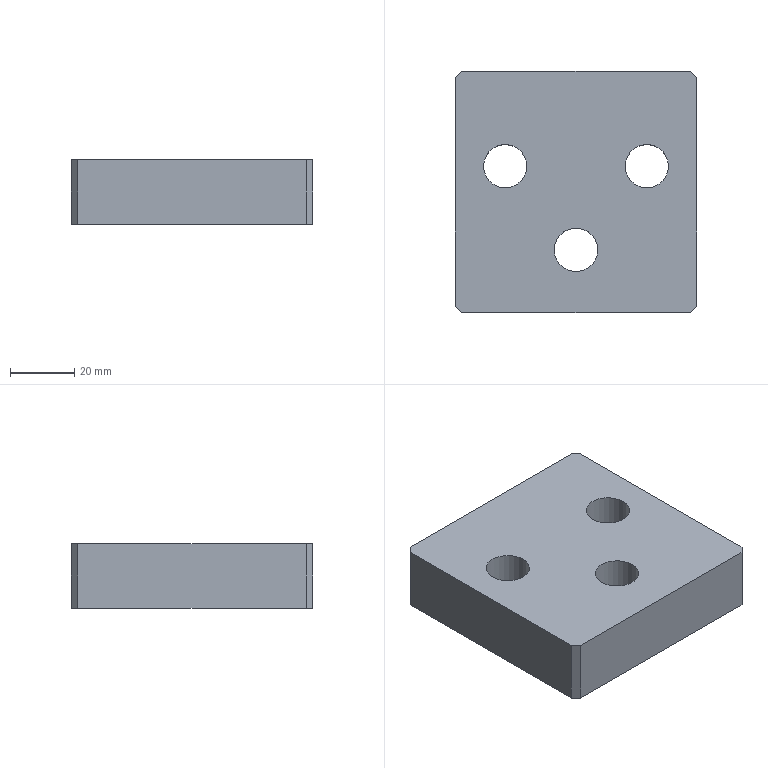Part | STEP file | lll_id1918_x_t | 1 solid | 13 faces | box 75 x 75 x 20 mm | volume 103740 mm3 | plane 10 | cylinder 3 | commonest cylinder face diameters 13.509 x3
STEP:
#1=CARTESIAN_POINT('',(3864.435,-427.,-98.5));
#2=VERTEX_POINT('',#1);
#3=CARTESIAN_POINT('',(3935.435,-427.,-98.5));
#4=VERTEX_POINT('',#3);
#5=CARTESIAN_POINT('',(3873.935,-427.,-98.5));
#6=DIRECTION('',(1.,0.,0.));
#7=VECTOR('',#6,1.);
#8=LINE('',#5,#7);
#9=EDGE_CURVE('',#2,#4,#8,.T.);
#10=ORIENTED_EDGE('',*,*,#9,.T.);
#11=CARTESIAN_POINT('',(3935.435,-427.,-78.5));
#12=VERTEX_POINT('',#11);
#13=CARTESIAN_POINT('',(3935.435,-427.,-78.5));
#14=DIRECTION('',(0.,0.,1.));
#15=VECTOR('',#14,1.);
#16=LINE('',#13,#15);
#17=EDGE_CURVE('',#4,#12,#16,.T.);
#18=ORIENTED_EDGE('',*,*,#17,.T.);
#19=CARTESIAN_POINT('',(3864.435,-427.,-78.5));
#20=VERTEX_POINT('',#19);
#21=CARTESIAN_POINT('',(3873.935,-427.,-78.5));
#22=DIRECTION('',(1.,0.,0.));
#23=VECTOR('',#22,1.);
#24=LINE('',#21,#23);
#25=EDGE_CURVE('',#20,#12,#24,.T.);
#26=ORIENTED_EDGE('',*,*,#25,.F.);
#27=CARTESIAN_POINT('',(3864.435,-427.,-78.5));
#28=DIRECTION('',(0.,0.,-1.));
#29=VECTOR('',#28,1.);
#30=LINE('',#27,#29);
#31=EDGE_CURVE('',#20,#2,#30,.T.);
#32=ORIENTED_EDGE('',*,*,#31,.T.);
#33=EDGE_LOOP('',(#10,#18,#26,#32));
#34=FACE_OUTER_BOUND('',#33,.T.);
#35=CARTESIAN_POINT('',(3873.935,-427.,-78.5));
#36=DIRECTION('',(0.,1.,0.));
#37=DIRECTION('',(0.,0.,1.));
#38=AXIS2_PLACEMENT_3D('',#35,#36,#37);
#39=PLANE('',#38);
#40=ADVANCED_FACE('',(#34),#39,.F.);
#41=CARTESIAN_POINT('',(3862.435,-354.,-78.5));
#42=VERTEX_POINT('',#41);
#43=CARTESIAN_POINT('',(3862.435,-425.,-78.5));
#44=VERTEX_POINT('',#43);
#45=CARTESIAN_POINT('',(3862.435,-362.5,-78.5));
#46=DIRECTION('',(0.,-1.,0.));
#47=VECTOR('',#46,1.);
#48=LINE('',#45,#47);
#49=EDGE_CURVE('',#42,#44,#48,.T.);
#50=ORIENTED_EDGE('',*,*,#49,.F.);
#51=CARTESIAN_POINT('',(3862.435,-354.,-98.5));
#52=VERTEX_POINT('',#51);
#53=CARTESIAN_POINT('',(3862.435,-354.,-78.5));
#54=DIRECTION('',(0.,0.,-1.));
#55=VECTOR('',#54,1.);
#56=LINE('',#53,#55);
#57=EDGE_CURVE('',#42,#52,#56,.T.);
#58=ORIENTED_EDGE('',*,*,#57,.T.);
#59=CARTESIAN_POINT('',(3862.435,-425.,-98.5));
#60=VERTEX_POINT('',#59);
#61=CARTESIAN_POINT('',(3862.435,-362.5,-98.5));
#62=DIRECTION('',(0.,-1.,0.));
#63=VECTOR('',#62,1.);
#64=LINE('',#61,#63);
#65=EDGE_CURVE('',#52,#60,#64,.T.);
#66=ORIENTED_EDGE('',*,*,#65,.T.);
#67=CARTESIAN_POINT('',(3862.435,-425.,-78.5));
#68=DIRECTION('',(0.,0.,1.));
#69=VECTOR('',#68,1.);
#70=LINE('',#67,#69);
#71=EDGE_CURVE('',#60,#44,#70,.T.);
#72=ORIENTED_EDGE('',*,*,#71,.T.);
#73=EDGE_LOOP('',(#50,#58,#66,#72));
#74=FACE_OUTER_BOUND('',#73,.T.);
#75=CARTESIAN_POINT('',(3862.435,-362.5,-78.5));
#76=DIRECTION('',(1.,0.,0.));
#77=DIRECTION('',(0.,0.,-1.));
#78=AXIS2_PLACEMENT_3D('',#75,#76,#77);
#79=PLANE('',#78);
#80=ADVANCED_FACE('',(#74),#79,.F.);
#81=CARTESIAN_POINT('',(3935.435,-352.,-78.5));
#82=VERTEX_POINT('',#81);
#83=CARTESIAN_POINT('',(3864.435,-352.,-78.5));
#84=VERTEX_POINT('',#83);
#85=CARTESIAN_POINT('',(3925.935,-352.,-78.5));
#86=DIRECTION('',(-1.,0.,0.));
#87=VECTOR('',#86,1.);
#88=LINE('',#85,#87);
#89=EDGE_CURVE('',#82,#84,#88,.T.);
#90=ORIENTED_EDGE('',*,*,#89,.F.);
#91=CARTESIAN_POINT('',(3935.435,-352.,-98.5));
#92=VERTEX_POINT('',#91);
#93=CARTESIAN_POINT('',(3935.435,-352.,-78.5));
#94=DIRECTION('',(0.,0.,-1.));
#95=VECTOR('',#94,1.);
#96=LINE('',#93,#95);
#97=EDGE_CURVE('',#82,#92,#96,.T.);
#98=ORIENTED_EDGE('',*,*,#97,.T.);
#99=CARTESIAN_POINT('',(3864.435,-352.,-98.5));
#100=VERTEX_POINT('',#99);
#101=CARTESIAN_POINT('',(3925.935,-352.,-98.5));
#102=DIRECTION('',(-1.,0.,0.));
#103=VECTOR('',#102,1.);
#104=LINE('',#101,#103);
#105=EDGE_CURVE('',#92,#100,#104,.T.);
#106=ORIENTED_EDGE('',*,*,#105,.T.);
#107=CARTESIAN_POINT('',(3864.435,-352.,-78.5));
#108=DIRECTION('',(0.,0.,1.));
#109=VECTOR('',#108,1.);
#110=LINE('',#107,#109);
#111=EDGE_CURVE('',#100,#84,#110,.T.);
#112=ORIENTED_EDGE('',*,*,#111,.T.);
#113=EDGE_LOOP('',(#90,#98,#106,#112));
#114=FACE_OUTER_BOUND('',#113,.T.);
#115=CARTESIAN_POINT('',(3925.935,-352.,-78.5));
#116=DIRECTION('',(0.,-1.,0.));
#117=DIRECTION('',(0.,0.,-1.));
#118=AXIS2_PLACEMENT_3D('',#115,#116,#117);
#119=PLANE('',#118);
#120=ADVANCED_FACE('',(#114),#119,.F.);
#121=CARTESIAN_POINT('',(3937.435,-425.,-78.5));
#122=VERTEX_POINT('',#121);
#123=CARTESIAN_POINT('',(3937.435,-354.,-78.5));
#124=VERTEX_POINT('',#123);
#125=CARTESIAN_POINT('',(3937.435,-411.5,-78.5));
#126=DIRECTION('',(0.,1.,0.));
#127=VECTOR('',#126,1.);
#128=LINE('',#125,#127);
#129=EDGE_CURVE('',#122,#124,#128,.T.);
#130=ORIENTED_EDGE('',*,*,#129,.F.);
#131=CARTESIAN_POINT('',(3937.435,-425.,-98.5));
#132=VERTEX_POINT('',#131);
#133=CARTESIAN_POINT('',(3937.435,-425.,-78.5));
#134=DIRECTION('',(0.,0.,-1.));
#135=VECTOR('',#134,1.);
#136=LINE('',#133,#135);
#137=EDGE_CURVE('',#122,#132,#136,.T.);
#138=ORIENTED_EDGE('',*,*,#137,.T.);
#139=CARTESIAN_POINT('',(3937.435,-354.,-98.5));
#140=VERTEX_POINT('',#139);
#141=CARTESIAN_POINT('',(3937.435,-411.5,-98.5));
#142=DIRECTION('',(0.,1.,0.));
#143=VECTOR('',#142,1.);
#144=LINE('',#141,#143);
#145=EDGE_CURVE('',#132,#140,#144,.T.);
#146=ORIENTED_EDGE('',*,*,#145,.T.);
#147=CARTESIAN_POINT('',(3937.435,-354.,-78.5));
#148=DIRECTION('',(0.,0.,1.));
#149=VECTOR('',#148,1.);
#150=LINE('',#147,#149);
#151=EDGE_CURVE('',#140,#124,#150,.T.);
#152=ORIENTED_EDGE('',*,*,#151,.T.);
#153=EDGE_LOOP('',(#130,#138,#146,#152));
#154=FACE_OUTER_BOUND('',#153,.T.);
#155=CARTESIAN_POINT('',(3937.435,-411.5,-78.5));
#156=DIRECTION('',(-1.,0.,0.));
#157=DIRECTION('',(0.,0.,1.));
#158=AXIS2_PLACEMENT_3D('',#155,#156,#157);
#159=PLANE('',#158);
#160=ADVANCED_FACE('',(#154),#159,.F.);
#161=CARTESIAN_POINT('',(3915.181,-381.5,-98.5));
#162=VERTEX_POINT('',#161);
#163=CARTESIAN_POINT('',(3921.935,-381.5,-98.5));
#164=DIRECTION('',(0.,0.,1.));
#165=DIRECTION('',(-1.,0.,0.));
#166=AXIS2_PLACEMENT_3D('',#163,#164,#165);
#167=CIRCLE('',#166,6.755);
#168=EDGE_CURVE('',#162,#162,#167,.T.);
#169=ORIENTED_EDGE('',*,*,#168,.T.);
#170=EDGE_LOOP('',(#169));
#171=FACE_BOUND('',#170,.T.);
#172=ORIENTED_EDGE('',*,*,#145,.F.);
#173=CARTESIAN_POINT('',(3937.435,-425.,-98.5));
#174=DIRECTION('',(-0.7071,-0.7071,0.));
#175=VECTOR('',#174,1.);
#176=LINE('',#173,#175);
#177=EDGE_CURVE('',#132,#4,#176,.T.);
#178=ORIENTED_EDGE('',*,*,#177,.T.);
#179=ORIENTED_EDGE('',*,*,#9,.F.);
#180=CARTESIAN_POINT('',(3864.435,-427.,-98.5));
#181=DIRECTION('',(-0.7071,0.7071,0.));
#182=VECTOR('',#181,1.);
#183=LINE('',#180,#182);
#184=EDGE_CURVE('',#2,#60,#183,.T.);
#185=ORIENTED_EDGE('',*,*,#184,.T.);
#186=ORIENTED_EDGE('',*,*,#65,.F.);
#187=CARTESIAN_POINT('',(3862.435,-354.,-98.5));
#188=DIRECTION('',(0.7071,0.7071,0.));
#189=VECTOR('',#188,1.);
#190=LINE('',#187,#189);
#191=EDGE_CURVE('',#52,#100,#190,.T.);
#192=ORIENTED_EDGE('',*,*,#191,.T.);
#193=ORIENTED_EDGE('',*,*,#105,.F.);
#194=CARTESIAN_POINT('',(3935.435,-352.,-98.5));
#195=DIRECTION('',(0.7071,-0.7071,0.));
#196=VECTOR('',#195,1.);
#197=LINE('',#194,#196);
#198=EDGE_CURVE('',#92,#140,#197,.T.);
#199=ORIENTED_EDGE('',*,*,#198,.T.);
#200=EDGE_LOOP('',(#172,#178,#179,#185,#186,#192,#193,#199));
#201=FACE_BOUND('',#200,.T.);
#202=CARTESIAN_POINT('',(3893.181,-407.5,-98.5));
#203=VERTEX_POINT('',#202);
#204=CARTESIAN_POINT('',(3899.935,-407.5,-98.5));
#205=DIRECTION('',(0.,0.,1.));
#206=DIRECTION('',(-1.,0.,0.));
#207=AXIS2_PLACEMENT_3D('',#204,#205,#206);
#208=CIRCLE('',#207,6.755);
#209=EDGE_CURVE('',#203,#203,#208,.T.);
#210=ORIENTED_EDGE('',*,*,#209,.T.);
#211=EDGE_LOOP('',(#210));
#212=FACE_BOUND('',#211,.T.);
#213=CARTESIAN_POINT('',(3871.181,-381.5,-98.5));
#214=VERTEX_POINT('',#213);
#215=CARTESIAN_POINT('',(3877.935,-381.5,-98.5));
#216=DIRECTION('',(0.,0.,1.));
#217=DIRECTION('',(-1.,0.,0.));
#218=AXIS2_PLACEMENT_3D('',#215,#216,#217);
#219=CIRCLE('',#218,6.755);
#220=EDGE_CURVE('',#214,#214,#219,.T.);
#221=ORIENTED_EDGE('',*,*,#220,.T.);
#222=EDGE_LOOP('',(#221));
#223=FACE_BOUND('',#222,.T.);
#224=CARTESIAN_POINT('',(3928.935,-359.5,-98.5));
#225=DIRECTION('',(0.,0.,1.));
#226=DIRECTION('',(1.,0.,0.));
#227=AXIS2_PLACEMENT_3D('',#224,#225,#226);
#228=PLANE('',#227);
#229=ADVANCED_FACE('',(#171,#201,#212,#223),#228,.F.);
#230=CARTESIAN_POINT('',(3915.181,-381.5,-78.5));
#231=VERTEX_POINT('',#230);
#232=CARTESIAN_POINT('',(3921.935,-381.5,-78.5));
#233=DIRECTION('',(0.,0.,1.));
#234=DIRECTION('',(-1.,0.,0.));
#235=AXIS2_PLACEMENT_3D('',#232,#233,#234);
#236=CIRCLE('',#235,6.755);
#237=EDGE_CURVE('',#231,#231,#236,.T.);
#238=ORIENTED_EDGE('',*,*,#237,.F.);
#239=EDGE_LOOP('',(#238));
#240=FACE_BOUND('',#239,.T.);
#241=ORIENTED_EDGE('',*,*,#25,.T.);
#242=CARTESIAN_POINT('',(3965.935,-396.5,-78.5));
#243=DIRECTION('',(0.7071,0.7071,0.));
#244=VECTOR('',#243,1.);
#245=LINE('',#242,#244);
#246=EDGE_CURVE('',#12,#122,#245,.T.);
#247=ORIENTED_EDGE('',*,*,#246,.T.);
#248=ORIENTED_EDGE('',*,*,#129,.T.);
#249=CARTESIAN_POINT('',(3938.435,-355.,-78.5));
#250=DIRECTION('',(-0.7071,0.7071,0.));
#251=VECTOR('',#250,1.);
#252=LINE('',#249,#251);
#253=EDGE_CURVE('',#124,#82,#252,.T.);
#254=ORIENTED_EDGE('',*,*,#253,.T.);
#255=ORIENTED_EDGE('',*,*,#89,.T.);
#256=CARTESIAN_POINT('',(3890.435,-326.,-78.5));
#257=DIRECTION('',(-0.7071,-0.7071,0.));
#258=VECTOR('',#257,1.);
#259=LINE('',#256,#258);
#260=EDGE_CURVE('',#84,#42,#259,.T.);
#261=ORIENTED_EDGE('',*,*,#260,.T.);
#262=ORIENTED_EDGE('',*,*,#49,.T.);
#263=CARTESIAN_POINT('',(3862.935,-425.5,-78.5));
#264=DIRECTION('',(0.7071,-0.7071,0.));
#265=VECTOR('',#264,1.);
#266=LINE('',#263,#265);
#267=EDGE_CURVE('',#44,#20,#266,.T.);
#268=ORIENTED_EDGE('',*,*,#267,.T.);
#269=EDGE_LOOP('',(#241,#247,#248,#254,#255,#261,#262,#268));
#270=FACE_BOUND('',#269,.T.);
#271=CARTESIAN_POINT('',(3893.181,-407.5,-78.5));
#272=VERTEX_POINT('',#271);
#273=CARTESIAN_POINT('',(3899.935,-407.5,-78.5));
#274=DIRECTION('',(0.,0.,1.));
#275=DIRECTION('',(-1.,0.,0.));
#276=AXIS2_PLACEMENT_3D('',#273,#274,#275);
#277=CIRCLE('',#276,6.755);
#278=EDGE_CURVE('',#272,#272,#277,.T.);
#279=ORIENTED_EDGE('',*,*,#278,.F.);
#280=EDGE_LOOP('',(#279));
#281=FACE_BOUND('',#280,.T.);
#282=CARTESIAN_POINT('',(3871.181,-381.5,-78.5));
#283=VERTEX_POINT('',#282);
#284=CARTESIAN_POINT('',(3877.935,-381.5,-78.5));
#285=DIRECTION('',(0.,0.,1.));
#286=DIRECTION('',(-1.,0.,0.));
#287=AXIS2_PLACEMENT_3D('',#284,#285,#286);
#288=CIRCLE('',#287,6.755);
#289=EDGE_CURVE('',#283,#283,#288,.T.);
#290=ORIENTED_EDGE('',*,*,#289,.F.);
#291=EDGE_LOOP('',(#290));
#292=FACE_BOUND('',#291,.T.);
#293=CARTESIAN_POINT('',(3928.935,-359.5,-78.5));
#294=DIRECTION('',(0.,0.,1.));
#295=DIRECTION('',(1.,0.,0.));
#296=AXIS2_PLACEMENT_3D('',#293,#294,#295);
#297=PLANE('',#296);
#298=ADVANCED_FACE('',(#240,#270,#281,#292),#297,.T.);
#299=ORIENTED_EDGE('',*,*,#278,.T.);
#300=EDGE_LOOP('',(#299));
#301=FACE_BOUND('',#300,.T.);
#302=ORIENTED_EDGE('',*,*,#209,.F.);
#303=EDGE_LOOP('',(#302));
#304=FACE_BOUND('',#303,.T.);
#305=CARTESIAN_POINT('',(3899.935,-407.5,89.5));
#306=DIRECTION('',(0.,0.,-1.));
#307=DIRECTION('',(-1.,0.,0.));
#308=AXIS2_PLACEMENT_3D('',#305,#306,#307);
#309=CYLINDRICAL_SURFACE('',#308,6.755);
#310=ADVANCED_FACE('',(#301,#304),#309,.F.);
#311=ORIENTED_EDGE('',*,*,#237,.T.);
#312=EDGE_LOOP('',(#311));
#313=FACE_BOUND('',#312,.T.);
#314=ORIENTED_EDGE('',*,*,#168,.F.);
#315=EDGE_LOOP('',(#314));
#316=FACE_BOUND('',#315,.T.);
#317=CARTESIAN_POINT('',(3921.935,-381.5,89.5));
#318=DIRECTION('',(0.,0.,-1.));
#319=DIRECTION('',(-1.,0.,0.));
#320=AXIS2_PLACEMENT_3D('',#317,#318,#319);
#321=CYLINDRICAL_SURFACE('',#320,6.755);
#322=ADVANCED_FACE('',(#313,#316),#321,.F.);
#323=ORIENTED_EDGE('',*,*,#289,.T.);
#324=EDGE_LOOP('',(#323));
#325=FACE_BOUND('',#324,.T.);
#326=ORIENTED_EDGE('',*,*,#220,.F.);
#327=EDGE_LOOP('',(#326));
#328=FACE_BOUND('',#327,.T.);
#329=CARTESIAN_POINT('',(3877.935,-381.5,89.5));
#330=DIRECTION('',(0.,0.,-1.));
#331=DIRECTION('',(-1.,0.,0.));
#332=AXIS2_PLACEMENT_3D('',#329,#330,#331);
#333=CYLINDRICAL_SURFACE('',#332,6.755);
#334=ADVANCED_FACE('',(#325,#328),#333,.F.);
#335=ORIENTED_EDGE('',*,*,#246,.F.);
#336=ORIENTED_EDGE('',*,*,#17,.F.);
#337=ORIENTED_EDGE('',*,*,#177,.F.);
#338=ORIENTED_EDGE('',*,*,#137,.F.);
#339=EDGE_LOOP('',(#335,#336,#337,#338));
#340=FACE_OUTER_BOUND('',#339,.T.);
#341=CARTESIAN_POINT('',(3937.435,-425.,-78.5));
#342=DIRECTION('',(-0.7071,0.7071,0.));
#343=DIRECTION('',(0.,0.,-1.));
#344=AXIS2_PLACEMENT_3D('',#341,#342,#343);
#345=PLANE('',#344);
#346=ADVANCED_FACE('',(#340),#345,.F.);
#347=ORIENTED_EDGE('',*,*,#253,.F.);
#348=ORIENTED_EDGE('',*,*,#151,.F.);
#349=ORIENTED_EDGE('',*,*,#198,.F.);
#350=ORIENTED_EDGE('',*,*,#97,.F.);
#351=EDGE_LOOP('',(#347,#348,#349,#350));
#352=FACE_OUTER_BOUND('',#351,.T.);
#353=CARTESIAN_POINT('',(3935.435,-352.,-78.5));
#354=DIRECTION('',(-0.7071,-0.7071,0.));
#355=DIRECTION('',(0.,0.,-1.));
#356=AXIS2_PLACEMENT_3D('',#353,#354,#355);
#357=PLANE('',#356);
#358=ADVANCED_FACE('',(#352),#357,.F.);
#359=ORIENTED_EDGE('',*,*,#260,.F.);
#360=ORIENTED_EDGE('',*,*,#111,.F.);
#361=ORIENTED_EDGE('',*,*,#191,.F.);
#362=ORIENTED_EDGE('',*,*,#57,.F.);
#363=EDGE_LOOP('',(#359,#360,#361,#362));
#364=FACE_OUTER_BOUND('',#363,.T.);
#365=CARTESIAN_POINT('',(3862.435,-354.,-78.5));
#366=DIRECTION('',(0.7071,-0.7071,0.));
#367=DIRECTION('',(0.,0.,-1.));
#368=AXIS2_PLACEMENT_3D('',#365,#366,#367);
#369=PLANE('',#368);
#370=ADVANCED_FACE('',(#364),#369,.F.);
#371=ORIENTED_EDGE('',*,*,#267,.F.);
#372=ORIENTED_EDGE('',*,*,#71,.F.);
#373=ORIENTED_EDGE('',*,*,#184,.F.);
#374=ORIENTED_EDGE('',*,*,#31,.F.);
#375=EDGE_LOOP('',(#371,#372,#373,#374));
#376=FACE_OUTER_BOUND('',#375,.T.);
#377=CARTESIAN_POINT('',(3864.435,-427.,-78.5));
#378=DIRECTION('',(0.7071,0.7071,0.));
#379=DIRECTION('',(0.,0.,-1.));
#380=AXIS2_PLACEMENT_3D('',#377,#378,#379);
#381=PLANE('',#380);
#382=ADVANCED_FACE('',(#376),#381,.F.);
#383=CLOSED_SHELL('',(#40,#80,#120,#160,#229,#298,#310,#322,#334,#346,#358,#370,#382));
#384=MANIFOLD_SOLID_BREP('',#383);
#385=(LENGTH_UNIT()NAMED_UNIT(*)SI_UNIT(.MILLI.,.METRE.));
#386=UNCERTAINTY_MEASURE_WITH_UNIT(LENGTH_MEASURE(0.00002),#385,'','');
#387=(NAMED_UNIT(*)PLANE_ANGLE_UNIT()SI_UNIT($,.RADIAN.));
#388=PLANE_ANGLE_MEASURE_WITH_UNIT(PLANE_ANGLE_MEASURE(0.01745),#387);
#389=DIMENSIONAL_EXPONENTS(0.,0.,0.,0.,0.,0.,0.);
#390=(CONVERSION_BASED_UNIT('DEGREE',#388)NAMED_UNIT(#389)PLANE_ANGLE_UNIT());
#391=(NAMED_UNIT(*)SI_UNIT($,.STERADIAN.)SOLID_ANGLE_UNIT());
#392=(GEOMETRIC_REPRESENTATION_CONTEXT(3)GLOBAL_UNCERTAINTY_ASSIGNED_CONTEXT((#386))GLOBAL_UNIT_ASSIGNED_CONTEXT((#385,#390,#391))REPRESENTATION_CONTEXT('',''));
#393=ADVANCED_BREP_SHAPE_REPRESENTATION('',(#384),#392);